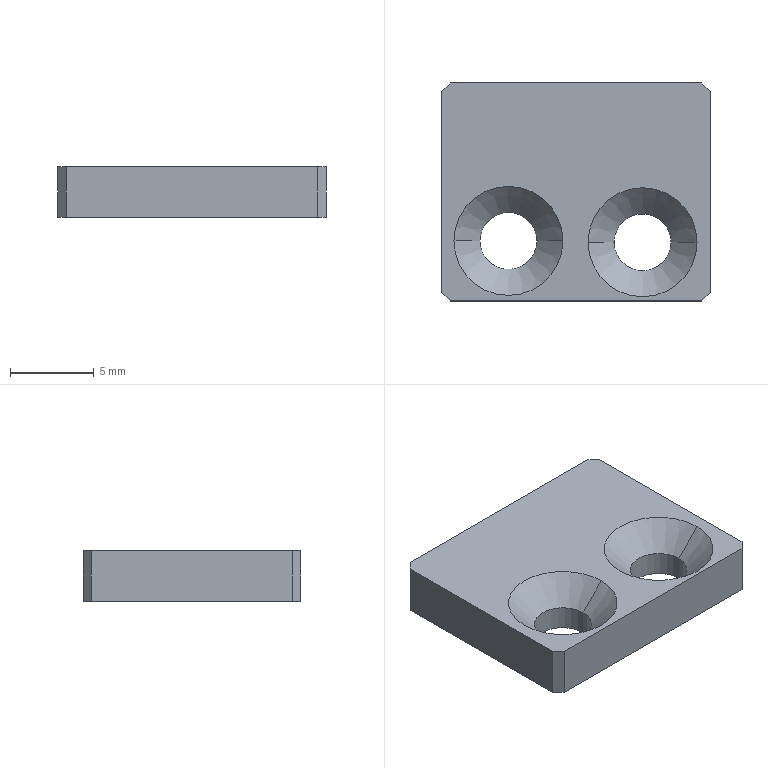Part | STEP file | 1 solid | 18 faces | box 16 x 13 x 3 mm | volume 534.563 mm3 | plane 10 | cone 4 | cylinder 4 | commonest cylinder face diameters 3.4 x4
STEP:
#1=CARTESIAN_POINT('',(0.,0.,0.));
#2=DIRECTION('',(0.,0.,1.));
#3=DIRECTION('',(1.,0.,0.));
#4=AXIS2_PLACEMENT_3D('',#1,#2,#3);
#5=CARTESIAN_POINT('',(7.5,-6.5,3.));
#6=VERTEX_POINT('',#5);
#7=CARTESIAN_POINT('',(8.,-6.,3.));
#8=VERTEX_POINT('',#7);
#9=CARTESIAN_POINT('',(8.,-6.,3.));
#10=DIRECTION('',(0.7071,0.7071,0.));
#11=VECTOR('',#10,1.);
#12=LINE('',#9,#11);
#13=CARTESIAN_POINT('',(8.,-6.,3.));
#14=DIRECTION('',(-0.7071,0.7071,0.));
#15=DIRECTION('',(0.,0.,-1.));
#16=AXIS2_PLACEMENT_3D('',#13,#14,#15);
#17=PLANE('',#16);
#18=CARTESIAN_POINT('',(0.,0.));
#19=DIRECTION('',(0.,-1.));
#20=VECTOR('',#19,1.);
#21=LINE('',#18,#20);
#22=(GEOMETRIC_REPRESENTATION_CONTEXT(2)PARAMETRIC_REPRESENTATION_CONTEXT()REPRESENTATION_CONTEXT('',''));
#23=DEFINITIONAL_REPRESENTATION('',(#21),#22);
#24=PCURVE('',#17,#23);
#25=CARTESIAN_POINT('',(0.,0.,3.));
#26=DIRECTION('',(0.,0.,-1.));
#27=DIRECTION('',(-1.,0.,0.));
#28=AXIS2_PLACEMENT_3D('',#25,#26,#27);
#29=PLANE('',#28);
#30=CARTESIAN_POINT('',(-8.,-6.));
#31=DIRECTION('',(-0.7071,0.7071));
#32=VECTOR('',#31,1.);
#33=LINE('',#30,#32);
#34=(GEOMETRIC_REPRESENTATION_CONTEXT(2)PARAMETRIC_REPRESENTATION_CONTEXT()REPRESENTATION_CONTEXT('',''));
#35=DEFINITIONAL_REPRESENTATION('',(#33),#34);
#36=PCURVE('',#29,#35);
#37=SURFACE_CURVE('',#12,(#24,#36),.PCURVE_S1.);
#38=EDGE_CURVE('',#6,#8,#37,.T.);
#39=ORIENTED_EDGE('',*,*,#38,.F.);
#40=CARTESIAN_POINT('',(7.5,-6.5,0.));
#41=VERTEX_POINT('',#40);
#42=CARTESIAN_POINT('',(7.5,-6.5,3.));
#43=DIRECTION('',(0.,0.,1.));
#44=VECTOR('',#43,1.);
#45=LINE('',#42,#44);
#46=CARTESIAN_POINT('',(0.,0.7071));
#47=DIRECTION('',(-1.,0.));
#48=VECTOR('',#47,1.);
#49=LINE('',#46,#48);
#50=(GEOMETRIC_REPRESENTATION_CONTEXT(2)PARAMETRIC_REPRESENTATION_CONTEXT()REPRESENTATION_CONTEXT('',''));
#51=DEFINITIONAL_REPRESENTATION('',(#49),#50);
#52=PCURVE('',#17,#51);
#53=CARTESIAN_POINT('',(-8.,-6.5,3.));
#54=DIRECTION('',(0.,1.,0.));
#55=DIRECTION('',(0.,0.,1.));
#56=AXIS2_PLACEMENT_3D('',#53,#54,#55);
#57=PLANE('',#56);
#58=CARTESIAN_POINT('',(0.,15.5));
#59=DIRECTION('',(1.,0.));
#60=VECTOR('',#59,1.);
#61=LINE('',#58,#60);
#62=(GEOMETRIC_REPRESENTATION_CONTEXT(2)PARAMETRIC_REPRESENTATION_CONTEXT()REPRESENTATION_CONTEXT('',''));
#63=DEFINITIONAL_REPRESENTATION('',(#61),#62);
#64=PCURVE('',#57,#63);
#65=SURFACE_CURVE('',#45,(#52,#64),.PCURVE_S1.);
#66=EDGE_CURVE('',#41,#6,#65,.T.);
#67=ORIENTED_EDGE('',*,*,#66,.F.);
#68=CARTESIAN_POINT('',(8.,-6.,0.));
#69=VERTEX_POINT('',#68);
#70=CARTESIAN_POINT('',(7.,-7.,0.));
#71=DIRECTION('',(-0.7071,-0.7071,0.));
#72=VECTOR('',#71,1.);
#73=LINE('',#70,#72);
#74=CARTESIAN_POINT('',(3.,1.414));
#75=DIRECTION('',(0.,1.));
#76=VECTOR('',#75,1.);
#77=LINE('',#74,#76);
#78=(GEOMETRIC_REPRESENTATION_CONTEXT(2)PARAMETRIC_REPRESENTATION_CONTEXT()REPRESENTATION_CONTEXT('',''));
#79=DEFINITIONAL_REPRESENTATION('',(#77),#78);
#80=PCURVE('',#17,#79);
#81=CARTESIAN_POINT('',(0.,0.,0.));
#82=DIRECTION('',(0.,0.,-1.));
#83=DIRECTION('',(-1.,0.,0.));
#84=AXIS2_PLACEMENT_3D('',#81,#82,#83);
#85=PLANE('',#84);
#86=CARTESIAN_POINT('',(-7.,-7.));
#87=DIRECTION('',(0.7071,-0.7071));
#88=VECTOR('',#87,1.);
#89=LINE('',#86,#88);
#90=(GEOMETRIC_REPRESENTATION_CONTEXT(2)PARAMETRIC_REPRESENTATION_CONTEXT()REPRESENTATION_CONTEXT('',''));
#91=DEFINITIONAL_REPRESENTATION('',(#89),#90);
#92=PCURVE('',#85,#91);
#93=SURFACE_CURVE('',#73,(#80,#92),.PCURVE_S1.);
#94=EDGE_CURVE('',#69,#41,#93,.T.);
#95=ORIENTED_EDGE('',*,*,#94,.F.);
#96=CARTESIAN_POINT('',(8.,-6.,3.));
#97=DIRECTION('',(0.,0.,-1.));
#98=VECTOR('',#97,1.);
#99=LINE('',#96,#98);
#100=CARTESIAN_POINT('',(0.,0.));
#101=DIRECTION('',(1.,0.));
#102=VECTOR('',#101,1.);
#103=LINE('',#100,#102);
#104=(GEOMETRIC_REPRESENTATION_CONTEXT(2)PARAMETRIC_REPRESENTATION_CONTEXT()REPRESENTATION_CONTEXT('',''));
#105=DEFINITIONAL_REPRESENTATION('',(#103),#104);
#106=PCURVE('',#17,#105);
#107=CARTESIAN_POINT('',(8.,-6.5,3.));
#108=DIRECTION('',(-1.,0.,0.));
#109=DIRECTION('',(0.,0.,1.));
#110=AXIS2_PLACEMENT_3D('',#107,#108,#109);
#111=PLANE('',#110);
#112=CARTESIAN_POINT('',(0.,0.5));
#113=DIRECTION('',(-1.,0.));
#114=VECTOR('',#113,1.);
#115=LINE('',#112,#114);
#116=(GEOMETRIC_REPRESENTATION_CONTEXT(2)PARAMETRIC_REPRESENTATION_CONTEXT()REPRESENTATION_CONTEXT('',''));
#117=DEFINITIONAL_REPRESENTATION('',(#115),#116);
#118=PCURVE('',#111,#117);
#119=SURFACE_CURVE('',#99,(#106,#118),.PCURVE_S1.);
#120=EDGE_CURVE('',#8,#69,#119,.T.);
#121=ORIENTED_EDGE('',*,*,#120,.F.);
#122=EDGE_LOOP('',(#39,#67,#95,#121));
#123=FACE_BOUND('',#122,.T.);
#124=ADVANCED_FACE('',(#123),#17,.F.);
#125=CARTESIAN_POINT('',(-8.,-6.,3.));
#126=VERTEX_POINT('',#125);
#127=CARTESIAN_POINT('',(-7.5,-6.5,3.));
#128=VERTEX_POINT('',#127);
#129=CARTESIAN_POINT('',(-7.5,-6.5,3.));
#130=DIRECTION('',(0.7071,-0.7071,0.));
#131=VECTOR('',#130,1.);
#132=LINE('',#129,#131);
#133=CARTESIAN_POINT('',(-7.5,-6.5,3.));
#134=DIRECTION('',(0.7071,0.7071,0.));
#135=DIRECTION('',(0.,0.,-1.));
#136=AXIS2_PLACEMENT_3D('',#133,#134,#135);
#137=PLANE('',#136);
#138=CARTESIAN_POINT('',(0.,0.));
#139=DIRECTION('',(0.,-1.));
#140=VECTOR('',#139,1.);
#141=LINE('',#138,#140);
#142=(GEOMETRIC_REPRESENTATION_CONTEXT(2)PARAMETRIC_REPRESENTATION_CONTEXT()REPRESENTATION_CONTEXT('',''));
#143=DEFINITIONAL_REPRESENTATION('',(#141),#142);
#144=PCURVE('',#137,#143);
#145=CARTESIAN_POINT('',(7.5,-6.5));
#146=DIRECTION('',(-0.7071,-0.7071));
#147=VECTOR('',#146,1.);
#148=LINE('',#145,#147);
#149=(GEOMETRIC_REPRESENTATION_CONTEXT(2)PARAMETRIC_REPRESENTATION_CONTEXT()REPRESENTATION_CONTEXT('',''));
#150=DEFINITIONAL_REPRESENTATION('',(#148),#149);
#151=PCURVE('',#29,#150);
#152=SURFACE_CURVE('',#132,(#144,#151),.PCURVE_S1.);
#153=EDGE_CURVE('',#126,#128,#152,.T.);
#154=ORIENTED_EDGE('',*,*,#153,.F.);
#155=CARTESIAN_POINT('',(-8.,-6.,0.));
#156=VERTEX_POINT('',#155);
#157=CARTESIAN_POINT('',(-8.,-6.,3.));
#158=DIRECTION('',(0.,0.,1.));
#159=VECTOR('',#158,1.);
#160=LINE('',#157,#159);
#161=CARTESIAN_POINT('',(0.,0.7071));
#162=DIRECTION('',(-1.,0.));
#163=VECTOR('',#162,1.);
#164=LINE('',#161,#163);
#165=(GEOMETRIC_REPRESENTATION_CONTEXT(2)PARAMETRIC_REPRESENTATION_CONTEXT()REPRESENTATION_CONTEXT('',''));
#166=DEFINITIONAL_REPRESENTATION('',(#164),#165);
#167=PCURVE('',#137,#166);
#168=CARTESIAN_POINT('',(-8.,-6.5,3.));
#169=DIRECTION('',(1.,0.,0.));
#170=DIRECTION('',(0.,0.,-1.));
#171=AXIS2_PLACEMENT_3D('',#168,#169,#170);
#172=PLANE('',#171);
#173=CARTESIAN_POINT('',(0.,0.5));
#174=DIRECTION('',(-1.,0.));
#175=VECTOR('',#174,1.);
#176=LINE('',#173,#175);
#177=(GEOMETRIC_REPRESENTATION_CONTEXT(2)PARAMETRIC_REPRESENTATION_CONTEXT()REPRESENTATION_CONTEXT('',''));
#178=DEFINITIONAL_REPRESENTATION('',(#176),#177);
#179=PCURVE('',#172,#178);
#180=SURFACE_CURVE('',#160,(#167,#179),.PCURVE_S1.);
#181=EDGE_CURVE('',#156,#126,#180,.T.);
#182=ORIENTED_EDGE('',*,*,#181,.F.);
#183=CARTESIAN_POINT('',(-7.5,-6.5,0.));
#184=VERTEX_POINT('',#183);
#185=CARTESIAN_POINT('',(-7.,-7.,0.));
#186=DIRECTION('',(-0.7071,0.7071,0.));
#187=VECTOR('',#186,1.);
#188=LINE('',#185,#187);
#189=CARTESIAN_POINT('',(3.,-0.7071));
#190=DIRECTION('',(0.,1.));
#191=VECTOR('',#190,1.);
#192=LINE('',#189,#191);
#193=(GEOMETRIC_REPRESENTATION_CONTEXT(2)PARAMETRIC_REPRESENTATION_CONTEXT()REPRESENTATION_CONTEXT('',''));
#194=DEFINITIONAL_REPRESENTATION('',(#192),#193);
#195=PCURVE('',#137,#194);
#196=CARTESIAN_POINT('',(7.,-7.));
#197=DIRECTION('',(0.7071,0.7071));
#198=VECTOR('',#197,1.);
#199=LINE('',#196,#198);
#200=(GEOMETRIC_REPRESENTATION_CONTEXT(2)PARAMETRIC_REPRESENTATION_CONTEXT()REPRESENTATION_CONTEXT('',''));
#201=DEFINITIONAL_REPRESENTATION('',(#199),#200);
#202=PCURVE('',#85,#201);
#203=SURFACE_CURVE('',#188,(#195,#202),.PCURVE_S1.);
#204=EDGE_CURVE('',#184,#156,#203,.T.);
#205=ORIENTED_EDGE('',*,*,#204,.F.);
#206=CARTESIAN_POINT('',(-7.5,-6.5,3.));
#207=DIRECTION('',(0.,0.,-1.));
#208=VECTOR('',#207,1.);
#209=LINE('',#206,#208);
#210=CARTESIAN_POINT('',(0.,0.));
#211=DIRECTION('',(1.,0.));
#212=VECTOR('',#211,1.);
#213=LINE('',#210,#212);
#214=(GEOMETRIC_REPRESENTATION_CONTEXT(2)PARAMETRIC_REPRESENTATION_CONTEXT()REPRESENTATION_CONTEXT('',''));
#215=DEFINITIONAL_REPRESENTATION('',(#213),#214);
#216=PCURVE('',#137,#215);
#217=CARTESIAN_POINT('',(0.,0.5));
#218=DIRECTION('',(-1.,0.));
#219=VECTOR('',#218,1.);
#220=LINE('',#217,#219);
#221=(GEOMETRIC_REPRESENTATION_CONTEXT(2)PARAMETRIC_REPRESENTATION_CONTEXT()REPRESENTATION_CONTEXT('',''));
#222=DEFINITIONAL_REPRESENTATION('',(#220),#221);
#223=PCURVE('',#57,#222);
#224=SURFACE_CURVE('',#209,(#216,#223),.PCURVE_S1.);
#225=EDGE_CURVE('',#128,#184,#224,.T.);
#226=ORIENTED_EDGE('',*,*,#225,.F.);
#227=EDGE_LOOP('',(#154,#182,#205,#226));
#228=FACE_BOUND('',#227,.T.);
#229=ADVANCED_FACE('',(#228),#137,.F.);
#230=CARTESIAN_POINT('',(-7.5,6.5,3.));
#231=VERTEX_POINT('',#230);
#232=CARTESIAN_POINT('',(-8.,6.,3.));
#233=VERTEX_POINT('',#232);
#234=CARTESIAN_POINT('',(-8.,6.,3.));
#235=DIRECTION('',(-0.7071,-0.7071,0.));
#236=VECTOR('',#235,1.);
#237=LINE('',#234,#236);
#238=CARTESIAN_POINT('',(-8.,6.,3.));
#239=DIRECTION('',(0.7071,-0.7071,0.));
#240=DIRECTION('',(0.,0.,-1.));
#241=AXIS2_PLACEMENT_3D('',#238,#239,#240);
#242=PLANE('',#241);
#243=CARTESIAN_POINT('',(0.,0.));
#244=DIRECTION('',(0.,-1.));
#245=VECTOR('',#244,1.);
#246=LINE('',#243,#245);
#247=(GEOMETRIC_REPRESENTATION_CONTEXT(2)PARAMETRIC_REPRESENTATION_CONTEXT()REPRESENTATION_CONTEXT('',''));
#248=DEFINITIONAL_REPRESENTATION('',(#246),#247);
#249=PCURVE('',#242,#248);
#250=CARTESIAN_POINT('',(8.,6.));
#251=DIRECTION('',(0.7071,-0.7071));
#252=VECTOR('',#251,1.);
#253=LINE('',#250,#252);
#254=(GEOMETRIC_REPRESENTATION_CONTEXT(2)PARAMETRIC_REPRESENTATION_CONTEXT()REPRESENTATION_CONTEXT('',''));
#255=DEFINITIONAL_REPRESENTATION('',(#253),#254);
#256=PCURVE('',#29,#255);
#257=SURFACE_CURVE('',#237,(#249,#256),.PCURVE_S1.);
#258=EDGE_CURVE('',#231,#233,#257,.T.);
#259=ORIENTED_EDGE('',*,*,#258,.F.);
#260=CARTESIAN_POINT('',(-7.5,6.5,0.));
#261=VERTEX_POINT('',#260);
#262=CARTESIAN_POINT('',(-7.5,6.5,3.));
#263=DIRECTION('',(0.,0.,1.));
#264=VECTOR('',#263,1.);
#265=LINE('',#262,#264);
#266=CARTESIAN_POINT('',(0.,0.7071));
#267=DIRECTION('',(-1.,0.));
#268=VECTOR('',#267,1.);
#269=LINE('',#266,#268);
#270=(GEOMETRIC_REPRESENTATION_CONTEXT(2)PARAMETRIC_REPRESENTATION_CONTEXT()REPRESENTATION_CONTEXT('',''));
#271=DEFINITIONAL_REPRESENTATION('',(#269),#270);
#272=PCURVE('',#242,#271);
#273=CARTESIAN_POINT('',(-8.,6.5,3.));
#274=DIRECTION('',(0.,-1.,0.));
#275=DIRECTION('',(0.,0.,-1.));
#276=AXIS2_PLACEMENT_3D('',#273,#274,#275);
#277=PLANE('',#276);
#278=CARTESIAN_POINT('',(0.,0.5));
#279=DIRECTION('',(-1.,0.));
#280=VECTOR('',#279,1.);
#281=LINE('',#278,#280);
#282=(GEOMETRIC_REPRESENTATION_CONTEXT(2)PARAMETRIC_REPRESENTATION_CONTEXT()REPRESENTATION_CONTEXT('',''));
#283=DEFINITIONAL_REPRESENTATION('',(#281),#282);
#284=PCURVE('',#277,#283);
#285=SURFACE_CURVE('',#265,(#272,#284),.PCURVE_S1.);
#286=EDGE_CURVE('',#261,#231,#285,.T.);
#287=ORIENTED_EDGE('',*,*,#286,.F.);
#288=CARTESIAN_POINT('',(-8.,6.,0.));
#289=VERTEX_POINT('',#288);
#290=CARTESIAN_POINT('',(-7.,7.,0.));
#291=DIRECTION('',(0.7071,0.7071,0.));
#292=VECTOR('',#291,1.);
#293=LINE('',#290,#292);
#294=CARTESIAN_POINT('',(3.,1.414));
#295=DIRECTION('',(0.,1.));
#296=VECTOR('',#295,1.);
#297=LINE('',#294,#296);
#298=(GEOMETRIC_REPRESENTATION_CONTEXT(2)PARAMETRIC_REPRESENTATION_CONTEXT()REPRESENTATION_CONTEXT('',''));
#299=DEFINITIONAL_REPRESENTATION('',(#297),#298);
#300=PCURVE('',#242,#299);
#301=CARTESIAN_POINT('',(7.,7.));
#302=DIRECTION('',(-0.7071,0.7071));
#303=VECTOR('',#302,1.);
#304=LINE('',#301,#303);
#305=(GEOMETRIC_REPRESENTATION_CONTEXT(2)PARAMETRIC_REPRESENTATION_CONTEXT()REPRESENTATION_CONTEXT('',''));
#306=DEFINITIONAL_REPRESENTATION('',(#304),#305);
#307=PCURVE('',#85,#306);
#308=SURFACE_CURVE('',#293,(#300,#307),.PCURVE_S1.);
#309=EDGE_CURVE('',#289,#261,#308,.T.);
#310=ORIENTED_EDGE('',*,*,#309,.F.);
#311=CARTESIAN_POINT('',(-8.,6.,3.));
#312=DIRECTION('',(0.,0.,-1.));
#313=VECTOR('',#312,1.);
#314=LINE('',#311,#313);
#315=CARTESIAN_POINT('',(0.,0.));
#316=DIRECTION('',(1.,0.));
#317=VECTOR('',#316,1.);
#318=LINE('',#315,#317);
#319=(GEOMETRIC_REPRESENTATION_CONTEXT(2)PARAMETRIC_REPRESENTATION_CONTEXT()REPRESENTATION_CONTEXT('',''));
#320=DEFINITIONAL_REPRESENTATION('',(#318),#319);
#321=PCURVE('',#242,#320);
#322=CARTESIAN_POINT('',(0.,12.5));
#323=DIRECTION('',(1.,0.));
#324=VECTOR('',#323,1.);
#325=LINE('',#322,#324);
#326=(GEOMETRIC_REPRESENTATION_CONTEXT(2)PARAMETRIC_REPRESENTATION_CONTEXT()REPRESENTATION_CONTEXT('',''));
#327=DEFINITIONAL_REPRESENTATION('',(#325),#326);
#328=PCURVE('',#172,#327);
#329=SURFACE_CURVE('',#314,(#321,#328),.PCURVE_S1.);
#330=EDGE_CURVE('',#233,#289,#329,.T.);
#331=ORIENTED_EDGE('',*,*,#330,.F.);
#332=EDGE_LOOP('',(#259,#287,#310,#331));
#333=FACE_BOUND('',#332,.T.);
#334=ADVANCED_FACE('',(#333),#242,.F.);
#335=CARTESIAN_POINT('',(8.,6.,3.));
#336=VERTEX_POINT('',#335);
#337=CARTESIAN_POINT('',(7.5,6.5,3.));
#338=VERTEX_POINT('',#337);
#339=CARTESIAN_POINT('',(7.5,6.5,3.));
#340=DIRECTION('',(-0.7071,0.7071,0.));
#341=VECTOR('',#340,1.);
#342=LINE('',#339,#341);
#343=CARTESIAN_POINT('',(7.5,6.5,3.));
#344=DIRECTION('',(-0.7071,-0.7071,0.));
#345=DIRECTION('',(0.,0.,-1.));
#346=AXIS2_PLACEMENT_3D('',#343,#344,#345);
#347=PLANE('',#346);
#348=CARTESIAN_POINT('',(0.,0.));
#349=DIRECTION('',(0.,-1.));
#350=VECTOR('',#349,1.);
#351=LINE('',#348,#350);
#352=(GEOMETRIC_REPRESENTATION_CONTEXT(2)PARAMETRIC_REPRESENTATION_CONTEXT()REPRESENTATION_CONTEXT('',''));
#353=DEFINITIONAL_REPRESENTATION('',(#351),#352);
#354=PCURVE('',#347,#353);
#355=CARTESIAN_POINT('',(-7.5,6.5));
#356=DIRECTION('',(0.7071,0.7071));
#357=VECTOR('',#356,1.);
#358=LINE('',#355,#357);
#359=(GEOMETRIC_REPRESENTATION_CONTEXT(2)PARAMETRIC_REPRESENTATION_CONTEXT()REPRESENTATION_CONTEXT('',''));
#360=DEFINITIONAL_REPRESENTATION('',(#358),#359);
#361=PCURVE('',#29,#360);
#362=SURFACE_CURVE('',#342,(#354,#361),.PCURVE_S1.);
#363=EDGE_CURVE('',#336,#338,#362,.T.);
#364=ORIENTED_EDGE('',*,*,#363,.F.);
#365=CARTESIAN_POINT('',(8.,6.,0.));
#366=VERTEX_POINT('',#365);
#367=CARTESIAN_POINT('',(8.,6.,3.));
#368=DIRECTION('',(0.,0.,1.));
#369=VECTOR('',#368,1.);
#370=LINE('',#367,#369);
#371=CARTESIAN_POINT('',(0.,0.7071));
#372=DIRECTION('',(-1.,0.));
#373=VECTOR('',#372,1.);
#374=LINE('',#371,#373);
#375=(GEOMETRIC_REPRESENTATION_CONTEXT(2)PARAMETRIC_REPRESENTATION_CONTEXT()REPRESENTATION_CONTEXT('',''));
#376=DEFINITIONAL_REPRESENTATION('',(#374),#375);
#377=PCURVE('',#347,#376);
#378=CARTESIAN_POINT('',(0.,12.5));
#379=DIRECTION('',(1.,0.));
#380=VECTOR('',#379,1.);
#381=LINE('',#378,#380);
#382=(GEOMETRIC_REPRESENTATION_CONTEXT(2)PARAMETRIC_REPRESENTATION_CONTEXT()REPRESENTATION_CONTEXT('',''));
#383=DEFINITIONAL_REPRESENTATION('',(#381),#382);
#384=PCURVE('',#111,#383);
#385=SURFACE_CURVE('',#370,(#377,#384),.PCURVE_S1.);
#386=EDGE_CURVE('',#366,#336,#385,.T.);
#387=ORIENTED_EDGE('',*,*,#386,.F.);
#388=CARTESIAN_POINT('',(7.5,6.5,0.));
#389=VERTEX_POINT('',#388);
#390=CARTESIAN_POINT('',(7.,7.,0.));
#391=DIRECTION('',(0.7071,-0.7071,0.));
#392=VECTOR('',#391,1.);
#393=LINE('',#390,#392);
#394=CARTESIAN_POINT('',(3.,-0.7071));
#395=DIRECTION('',(0.,1.));
#396=VECTOR('',#395,1.);
#397=LINE('',#394,#396);
#398=(GEOMETRIC_REPRESENTATION_CONTEXT(2)PARAMETRIC_REPRESENTATION_CONTEXT()REPRESENTATION_CONTEXT('',''));
#399=DEFINITIONAL_REPRESENTATION('',(#397),#398);
#400=PCURVE('',#347,#399);
#401=CARTESIAN_POINT('',(-7.,7.));
#402=DIRECTION('',(-0.7071,-0.7071));
#403=VECTOR('',#402,1.);
#404=LINE('',#401,#403);
#405=(GEOMETRIC_REPRESENTATION_CONTEXT(2)PARAMETRIC_REPRESENTATION_CONTEXT()REPRESENTATION_CONTEXT('',''));
#406=DEFINITIONAL_REPRESENTATION('',(#404),#405);
#407=PCURVE('',#85,#406);
#408=SURFACE_CURVE('',#393,(#400,#407),.PCURVE_S1.);
#409=EDGE_CURVE('',#389,#366,#408,.T.);
#410=ORIENTED_EDGE('',*,*,#409,.F.);
#411=CARTESIAN_POINT('',(7.5,6.5,3.));
#412=DIRECTION('',(0.,0.,-1.));
#413=VECTOR('',#412,1.);
#414=LINE('',#411,#413);
#415=CARTESIAN_POINT('',(0.,0.));
#416=DIRECTION('',(1.,0.));
#417=VECTOR('',#416,1.);
#418=LINE('',#415,#417);
#419=(GEOMETRIC_REPRESENTATION_CONTEXT(2)PARAMETRIC_REPRESENTATION_CONTEXT()REPRESENTATION_CONTEXT('',''));
#420=DEFINITIONAL_REPRESENTATION('',(#418),#419);
#421=PCURVE('',#347,#420);
#422=CARTESIAN_POINT('',(0.,15.5));
#423=DIRECTION('',(1.,0.));
#424=VECTOR('',#423,1.);
#425=LINE('',#422,#424);
#426=(GEOMETRIC_REPRESENTATION_CONTEXT(2)PARAMETRIC_REPRESENTATION_CONTEXT()REPRESENTATION_CONTEXT('',''));
#427=DEFINITIONAL_REPRESENTATION('',(#425),#426);
#428=PCURVE('',#277,#427);
#429=SURFACE_CURVE('',#414,(#421,#428),.PCURVE_S1.);
#430=EDGE_CURVE('',#338,#389,#429,.T.);
#431=ORIENTED_EDGE('',*,*,#430,.F.);
#432=EDGE_LOOP('',(#364,#387,#410,#431));
#433=FACE_BOUND('',#432,.T.);
#434=ADVANCED_FACE('',(#433),#347,.F.);
#435=CARTESIAN_POINT('',(-0.7797,-2.919,3.));
#436=VERTEX_POINT('',#435);
#437=CARTESIAN_POINT('',(-7.28,-2.919,3.));
#438=VERTEX_POINT('',#437);
#439=CARTESIAN_POINT('',(-4.03,-2.919,3.));
#440=DIRECTION('',(0.,0.,1.));
#441=DIRECTION('',(1.,0.,0.));
#442=AXIS2_PLACEMENT_3D('',#439,#440,#441);
#443=CIRCLE('',#442,3.25);
#444=CARTESIAN_POINT('',(-4.03,-2.919,3.));
#445=DIRECTION('',(0.,0.,1.));
#446=DIRECTION('',(1.,0.,0.));
#447=AXIS2_PLACEMENT_3D('',#444,#445,#446);
#448=CONICAL_SURFACE('',#447,3.25,0.7854);
#449=CARTESIAN_POINT('',(0.,0.));
#450=DIRECTION('',(1.,0.));
#451=VECTOR('',#450,1.);
#452=LINE('',#449,#451);
#453=(GEOMETRIC_REPRESENTATION_CONTEXT(2)PARAMETRIC_REPRESENTATION_CONTEXT()REPRESENTATION_CONTEXT('',''));
#454=DEFINITIONAL_REPRESENTATION('',(#452),#453);
#455=PCURVE('',#448,#454);
#456=CARTESIAN_POINT('',(0.7797,-2.919));
#457=CARTESIAN_POINT('',(0.7797,2.71));
#458=CARTESIAN_POINT('',(5.655,-0.1046));
#459=CARTESIAN_POINT('',(10.53,-2.919));
#460=CARTESIAN_POINT('',(5.655,-5.734));
#461=CARTESIAN_POINT('',(0.7797,-8.548));
#462=CARTESIAN_POINT('',(0.7797,-2.919));
#463=(BOUNDED_CURVE()B_SPLINE_CURVE(2,(#456,#457,#458,#459,#460,#461,#462),.UNSPECIFIED.,.T.,.F.)B_SPLINE_CURVE_WITH_KNOTS((1,2,2,2,2,1),(-2.094,0.,2.094,4.189,6.283,8.378),.UNSPECIFIED.)CURVE()GEOMETRIC_REPRESENTATION_ITEM()RATIONAL_B_SPLINE_CURVE((1.,0.5,1.,0.5,1.,0.5,1.))REPRESENTATION_ITEM(''));
#464=(GEOMETRIC_REPRESENTATION_CONTEXT(2)PARAMETRIC_REPRESENTATION_CONTEXT()REPRESENTATION_CONTEXT('',''));
#465=DEFINITIONAL_REPRESENTATION('',(#463),#464);
#466=PCURVE('',#29,#465);
#467=SURFACE_CURVE('',#443,(#455,#466),.PCURVE_S1.);
#468=EDGE_CURVE('',#436,#438,#467,.T.);
#469=ORIENTED_EDGE('',*,*,#468,.F.);
#470=CARTESIAN_POINT('',(-2.33,-2.919,1.45));
#471=VERTEX_POINT('',#470);
#472=CARTESIAN_POINT('',(-0.7797,-2.919,3.));
#473=DIRECTION('',(0.7071,0.,0.7071));
#474=VECTOR('',#473,1.);
#475=LINE('',#472,#474);
#476=CARTESIAN_POINT('',(0.,0.));
#477=DIRECTION('',(0.,1.));
#478=VECTOR('',#477,1.);
#479=LINE('',#476,#478);
#480=(GEOMETRIC_REPRESENTATION_CONTEXT(2)PARAMETRIC_REPRESENTATION_CONTEXT()REPRESENTATION_CONTEXT('',''));
#481=DEFINITIONAL_REPRESENTATION('',(#479),#480);
#482=PCURVE('',#448,#481);
#483=CARTESIAN_POINT('',(-4.03,-2.919,3.));
#484=DIRECTION('',(0.,0.,1.));
#485=DIRECTION('',(1.,0.,0.));
#486=AXIS2_PLACEMENT_3D('',#483,#484,#485);
#487=CONICAL_SURFACE('',#486,3.25,0.7854);
#488=CARTESIAN_POINT('',(6.283,0.));
#489=DIRECTION('',(0.,1.));
#490=VECTOR('',#489,1.);
#491=LINE('',#488,#490);
#492=(GEOMETRIC_REPRESENTATION_CONTEXT(2)PARAMETRIC_REPRESENTATION_CONTEXT()REPRESENTATION_CONTEXT('',''));
#493=DEFINITIONAL_REPRESENTATION('',(#491),#492);
#494=PCURVE('',#487,#493);
#495=SURFACE_CURVE('',#475,(#482,#494),.PCURVE_S1.);
#496=EDGE_CURVE('',#471,#436,#495,.T.);
#497=ORIENTED_EDGE('',*,*,#496,.F.);
#498=CARTESIAN_POINT('',(-5.73,-2.919,1.45));
#499=VERTEX_POINT('',#498);
#500=CARTESIAN_POINT('',(-4.03,-2.919,1.45));
#501=DIRECTION('',(0.,0.,1.));
#502=DIRECTION('',(1.,0.,0.));
#503=AXIS2_PLACEMENT_3D('',#500,#501,#502);
#504=CIRCLE('',#503,1.7);
#505=CARTESIAN_POINT('',(0.,-1.55));
#506=DIRECTION('',(1.,0.));
#507=VECTOR('',#506,1.);
#508=LINE('',#505,#507);
#509=(GEOMETRIC_REPRESENTATION_CONTEXT(2)PARAMETRIC_REPRESENTATION_CONTEXT()REPRESENTATION_CONTEXT('',''));
#510=DEFINITIONAL_REPRESENTATION('',(#508),#509);
#511=PCURVE('',#448,#510);
#512=CARTESIAN_POINT('',(-4.03,-2.919,3.));
#513=DIRECTION('',(0.,0.,1.));
#514=DIRECTION('',(1.,0.,0.));
#515=AXIS2_PLACEMENT_3D('',#512,#513,#514);
#516=CYLINDRICAL_SURFACE('',#515,1.7);
#517=CARTESIAN_POINT('',(0.,-1.55));
#518=DIRECTION('',(1.,0.));
#519=VECTOR('',#518,1.);
#520=LINE('',#517,#519);
#521=(GEOMETRIC_REPRESENTATION_CONTEXT(2)PARAMETRIC_REPRESENTATION_CONTEXT()REPRESENTATION_CONTEXT('',''));
#522=DEFINITIONAL_REPRESENTATION('',(#520),#521);
#523=PCURVE('',#516,#522);
#524=SURFACE_CURVE('',#504,(#511,#523),.PCURVE_S1.);
#525=EDGE_CURVE('',#471,#499,#524,.T.);
#526=ORIENTED_EDGE('',*,*,#525,.T.);
#527=CARTESIAN_POINT('',(-7.28,-2.919,3.));
#528=DIRECTION('',(-0.7071,0.,0.7071));
#529=VECTOR('',#528,1.);
#530=LINE('',#527,#529);
#531=CARTESIAN_POINT('',(3.142,0.));
#532=DIRECTION('',(0.,1.));
#533=VECTOR('',#532,1.);
#534=LINE('',#531,#533);
#535=(GEOMETRIC_REPRESENTATION_CONTEXT(2)PARAMETRIC_REPRESENTATION_CONTEXT()REPRESENTATION_CONTEXT('',''));
#536=DEFINITIONAL_REPRESENTATION('',(#534),#535);
#537=PCURVE('',#448,#536);
#538=CARTESIAN_POINT('',(3.142,0.));
#539=DIRECTION('',(0.,1.));
#540=VECTOR('',#539,1.);
#541=LINE('',#538,#540);
#542=(GEOMETRIC_REPRESENTATION_CONTEXT(2)PARAMETRIC_REPRESENTATION_CONTEXT()REPRESENTATION_CONTEXT('',''));
#543=DEFINITIONAL_REPRESENTATION('',(#541),#542);
#544=PCURVE('',#487,#543);
#545=SURFACE_CURVE('',#530,(#537,#544),.PCURVE_S1.);
#546=EDGE_CURVE('',#499,#438,#545,.T.);
#547=ORIENTED_EDGE('',*,*,#546,.T.);
#548=EDGE_LOOP('',(#469,#497,#526,#547));
#549=FACE_BOUND('',#548,.F.);
#550=ADVANCED_FACE('',(#549),#448,.F.);
#551=ORIENTED_EDGE('',*,*,#525,.F.);
#552=CARTESIAN_POINT('',(-2.33,-2.919,0.));
#553=VERTEX_POINT('',#552);
#554=CARTESIAN_POINT('',(-2.33,-2.919,3.));
#555=DIRECTION('',(0.,0.,1.));
#556=VECTOR('',#555,1.);
#557=LINE('',#554,#556);
#558=CARTESIAN_POINT('',(0.,0.));
#559=DIRECTION('',(0.,1.));
#560=VECTOR('',#559,1.);
#561=LINE('',#558,#560);
#562=(GEOMETRIC_REPRESENTATION_CONTEXT(2)PARAMETRIC_REPRESENTATION_CONTEXT()REPRESENTATION_CONTEXT('',''));
#563=DEFINITIONAL_REPRESENTATION('',(#561),#562);
#564=PCURVE('',#516,#563);
#565=CARTESIAN_POINT('',(-4.03,-2.919,3.));
#566=DIRECTION('',(0.,0.,1.));
#567=DIRECTION('',(1.,0.,0.));
#568=AXIS2_PLACEMENT_3D('',#565,#566,#567);
#569=CYLINDRICAL_SURFACE('',#568,1.7);
#570=CARTESIAN_POINT('',(6.283,0.));
#571=DIRECTION('',(0.,1.));
#572=VECTOR('',#571,1.);
#573=LINE('',#570,#572);
#574=(GEOMETRIC_REPRESENTATION_CONTEXT(2)PARAMETRIC_REPRESENTATION_CONTEXT()REPRESENTATION_CONTEXT('',''));
#575=DEFINITIONAL_REPRESENTATION('',(#573),#574);
#576=PCURVE('',#569,#575);
#577=SURFACE_CURVE('',#557,(#564,#576),.PCURVE_S1.);
#578=EDGE_CURVE('',#553,#471,#577,.T.);
#579=ORIENTED_EDGE('',*,*,#578,.F.);
#580=CARTESIAN_POINT('',(-5.73,-2.919,0.));
#581=VERTEX_POINT('',#580);
#582=CARTESIAN_POINT('',(-4.03,-2.919,0.));
#583=DIRECTION('',(0.,0.,1.));
#584=DIRECTION('',(1.,0.,0.));
#585=AXIS2_PLACEMENT_3D('',#582,#583,#584);
#586=CIRCLE('',#585,1.7);
#587=CARTESIAN_POINT('',(0.,-3.));
#588=DIRECTION('',(1.,0.));
#589=VECTOR('',#588,1.);
#590=LINE('',#587,#589);
#591=(GEOMETRIC_REPRESENTATION_CONTEXT(2)PARAMETRIC_REPRESENTATION_CONTEXT()REPRESENTATION_CONTEXT('',''));
#592=DEFINITIONAL_REPRESENTATION('',(#590),#591);
#593=PCURVE('',#516,#592);
#594=CARTESIAN_POINT('',(2.33,-2.919));
#595=CARTESIAN_POINT('',(2.33,0.02529));
#596=CARTESIAN_POINT('',(4.88,-1.447));
#597=CARTESIAN_POINT('',(7.43,-2.919));
#598=CARTESIAN_POINT('',(4.88,-4.391));
#599=CARTESIAN_POINT('',(2.33,-5.864));
#600=CARTESIAN_POINT('',(2.33,-2.919));
#601=(BOUNDED_CURVE()B_SPLINE_CURVE(2,(#594,#595,#596,#597,#598,#599,#600),.UNSPECIFIED.,.T.,.F.)B_SPLINE_CURVE_WITH_KNOTS((1,2,2,2,2,1),(-2.094,0.,2.094,4.189,6.283,8.378),.UNSPECIFIED.)CURVE()GEOMETRIC_REPRESENTATION_ITEM()RATIONAL_B_SPLINE_CURVE((1.,0.5,1.,0.5,1.,0.5,1.))REPRESENTATION_ITEM(''));
#602=(GEOMETRIC_REPRESENTATION_CONTEXT(2)PARAMETRIC_REPRESENTATION_CONTEXT()REPRESENTATION_CONTEXT('',''));
#603=DEFINITIONAL_REPRESENTATION('',(#601),#602);
#604=PCURVE('',#85,#603);
#605=SURFACE_CURVE('',#586,(#593,#604),.PCURVE_S1.);
#606=EDGE_CURVE('',#553,#581,#605,.T.);
#607=ORIENTED_EDGE('',*,*,#606,.T.);
#608=CARTESIAN_POINT('',(-5.73,-2.919,3.));
#609=DIRECTION('',(0.,0.,1.));
#610=VECTOR('',#609,1.);
#611=LINE('',#608,#610);
#612=CARTESIAN_POINT('',(3.142,0.));
#613=DIRECTION('',(0.,1.));
#614=VECTOR('',#613,1.);
#615=LINE('',#612,#614);
#616=(GEOMETRIC_REPRESENTATION_CONTEXT(2)PARAMETRIC_REPRESENTATION_CONTEXT()REPRESENTATION_CONTEXT('',''));
#617=DEFINITIONAL_REPRESENTATION('',(#615),#616);
#618=PCURVE('',#516,#617);
#619=CARTESIAN_POINT('',(3.142,0.));
#620=DIRECTION('',(0.,1.));
#621=VECTOR('',#620,1.);
#622=LINE('',#619,#621);
#623=(GEOMETRIC_REPRESENTATION_CONTEXT(2)PARAMETRIC_REPRESENTATION_CONTEXT()REPRESENTATION_CONTEXT('',''));
#624=DEFINITIONAL_REPRESENTATION('',(#622),#623);
#625=PCURVE('',#569,#624);
#626=SURFACE_CURVE('',#611,(#618,#625),.PCURVE_S1.);
#627=EDGE_CURVE('',#581,#499,#626,.T.);
#628=ORIENTED_EDGE('',*,*,#627,.T.);
#629=EDGE_LOOP('',(#551,#579,#607,#628));
#630=FACE_BOUND('',#629,.F.);
#631=ADVANCED_FACE('',(#630),#516,.F.);
#632=CARTESIAN_POINT('',(7.22,-3.,3.));
#633=VERTEX_POINT('',#632);
#634=CARTESIAN_POINT('',(0.7199,-3.,3.));
#635=VERTEX_POINT('',#634);
#636=CARTESIAN_POINT('',(3.97,-3.,3.));
#637=DIRECTION('',(0.,0.,1.));
#638=DIRECTION('',(1.,0.,0.));
#639=AXIS2_PLACEMENT_3D('',#636,#637,#638);
#640=CIRCLE('',#639,3.25);
#641=CARTESIAN_POINT('',(3.97,-3.,3.));
#642=DIRECTION('',(0.,0.,1.));
#643=DIRECTION('',(1.,0.,0.));
#644=AXIS2_PLACEMENT_3D('',#641,#642,#643);
#645=CONICAL_SURFACE('',#644,3.25,0.7854);
#646=CARTESIAN_POINT('',(0.,0.));
#647=DIRECTION('',(1.,0.));
#648=VECTOR('',#647,1.);
#649=LINE('',#646,#648);
#650=(GEOMETRIC_REPRESENTATION_CONTEXT(2)PARAMETRIC_REPRESENTATION_CONTEXT()REPRESENTATION_CONTEXT('',''));
#651=DEFINITIONAL_REPRESENTATION('',(#649),#650);
#652=PCURVE('',#645,#651);
#653=CARTESIAN_POINT('',(-7.22,-3.));
#654=CARTESIAN_POINT('',(-7.22,2.629));
#655=CARTESIAN_POINT('',(-2.345,-0.1854));
#656=CARTESIAN_POINT('',(2.53,-3.));
#657=CARTESIAN_POINT('',(-2.345,-5.815));
#658=CARTESIAN_POINT('',(-7.22,-8.629));
#659=CARTESIAN_POINT('',(-7.22,-3.));
#660=(BOUNDED_CURVE()B_SPLINE_CURVE(2,(#653,#654,#655,#656,#657,#658,#659),.UNSPECIFIED.,.T.,.F.)B_SPLINE_CURVE_WITH_KNOTS((1,2,2,2,2,1),(-2.094,0.,2.094,4.189,6.283,8.378),.UNSPECIFIED.)CURVE()GEOMETRIC_REPRESENTATION_ITEM()RATIONAL_B_SPLINE_CURVE((1.,0.5,1.,0.5,1.,0.5,1.))REPRESENTATION_ITEM(''));
#661=(GEOMETRIC_REPRESENTATION_CONTEXT(2)PARAMETRIC_REPRESENTATION_CONTEXT()REPRESENTATION_CONTEXT('',''));
#662=DEFINITIONAL_REPRESENTATION('',(#660),#661);
#663=PCURVE('',#29,#662);
#664=SURFACE_CURVE('',#640,(#652,#663),.PCURVE_S1.);
#665=EDGE_CURVE('',#633,#635,#664,.T.);
#666=ORIENTED_EDGE('',*,*,#665,.F.);
#667=CARTESIAN_POINT('',(5.67,-3.,1.45));
#668=VERTEX_POINT('',#667);
#669=CARTESIAN_POINT('',(7.22,-3.,3.));
#670=DIRECTION('',(0.7071,0.,0.7071));
#671=VECTOR('',#670,1.);
#672=LINE('',#669,#671);
#673=CARTESIAN_POINT('',(0.,0.));
#674=DIRECTION('',(0.,1.));
#675=VECTOR('',#674,1.);
#676=LINE('',#673,#675);
#677=(GEOMETRIC_REPRESENTATION_CONTEXT(2)PARAMETRIC_REPRESENTATION_CONTEXT()REPRESENTATION_CONTEXT('',''));
#678=DEFINITIONAL_REPRESENTATION('',(#676),#677);
#679=PCURVE('',#645,#678);
#680=CARTESIAN_POINT('',(3.97,-3.,3.));
#681=DIRECTION('',(0.,0.,1.));
#682=DIRECTION('',(1.,0.,0.));
#683=AXIS2_PLACEMENT_3D('',#680,#681,#682);
#684=CONICAL_SURFACE('',#683,3.25,0.7854);
#685=CARTESIAN_POINT('',(6.283,0.));
#686=DIRECTION('',(0.,1.));
#687=VECTOR('',#686,1.);
#688=LINE('',#685,#687);
#689=(GEOMETRIC_REPRESENTATION_CONTEXT(2)PARAMETRIC_REPRESENTATION_CONTEXT()REPRESENTATION_CONTEXT('',''));
#690=DEFINITIONAL_REPRESENTATION('',(#688),#689);
#691=PCURVE('',#684,#690);
#692=SURFACE_CURVE('',#672,(#679,#691),.PCURVE_S1.);
#693=EDGE_CURVE('',#668,#633,#692,.T.);
#694=ORIENTED_EDGE('',*,*,#693,.F.);
#695=CARTESIAN_POINT('',(2.27,-3.,1.45));
#696=VERTEX_POINT('',#695);
#697=CARTESIAN_POINT('',(3.97,-3.,1.45));
#698=DIRECTION('',(0.,0.,1.));
#699=DIRECTION('',(1.,0.,0.));
#700=AXIS2_PLACEMENT_3D('',#697,#698,#699);
#701=CIRCLE('',#700,1.7);
#702=CARTESIAN_POINT('',(0.,-1.55));
#703=DIRECTION('',(1.,0.));
#704=VECTOR('',#703,1.);
#705=LINE('',#702,#704);
#706=(GEOMETRIC_REPRESENTATION_CONTEXT(2)PARAMETRIC_REPRESENTATION_CONTEXT()REPRESENTATION_CONTEXT('',''));
#707=DEFINITIONAL_REPRESENTATION('',(#705),#706);
#708=PCURVE('',#645,#707);
#709=CARTESIAN_POINT('',(3.97,-3.,3.));
#710=DIRECTION('',(0.,0.,1.));
#711=DIRECTION('',(1.,0.,0.));
#712=AXIS2_PLACEMENT_3D('',#709,#710,#711);
#713=CYLINDRICAL_SURFACE('',#712,1.7);
#714=CARTESIAN_POINT('',(0.,-1.55));
#715=DIRECTION('',(1.,0.));
#716=VECTOR('',#715,1.);
#717=LINE('',#714,#716);
#718=(GEOMETRIC_REPRESENTATION_CONTEXT(2)PARAMETRIC_REPRESENTATION_CONTEXT()REPRESENTATION_CONTEXT('',''));
#719=DEFINITIONAL_REPRESENTATION('',(#717),#718);
#720=PCURVE('',#713,#719);
#721=SURFACE_CURVE('',#701,(#708,#720),.PCURVE_S1.);
#722=EDGE_CURVE('',#668,#696,#721,.T.);
#723=ORIENTED_EDGE('',*,*,#722,.T.);
#724=CARTESIAN_POINT('',(0.7199,-3.,3.));
#725=DIRECTION('',(-0.7071,0.,0.7071));
#726=VECTOR('',#725,1.);
#727=LINE('',#724,#726);
#728=CARTESIAN_POINT('',(3.142,0.));
#729=DIRECTION('',(0.,1.));
#730=VECTOR('',#729,1.);
#731=LINE('',#728,#730);
#732=(GEOMETRIC_REPRESENTATION_CONTEXT(2)PARAMETRIC_REPRESENTATION_CONTEXT()REPRESENTATION_CONTEXT('',''));
#733=DEFINITIONAL_REPRESENTATION('',(#731),#732);
#734=PCURVE('',#645,#733);
#735=CARTESIAN_POINT('',(3.142,0.));
#736=DIRECTION('',(0.,1.));
#737=VECTOR('',#736,1.);
#738=LINE('',#735,#737);
#739=(GEOMETRIC_REPRESENTATION_CONTEXT(2)PARAMETRIC_REPRESENTATION_CONTEXT()REPRESENTATION_CONTEXT('',''));
#740=DEFINITIONAL_REPRESENTATION('',(#738),#739);
#741=PCURVE('',#684,#740);
#742=SURFACE_CURVE('',#727,(#734,#741),.PCURVE_S1.);
#743=EDGE_CURVE('',#696,#635,#742,.T.);
#744=ORIENTED_EDGE('',*,*,#743,.T.);
#745=EDGE_LOOP('',(#666,#694,#723,#744));
#746=FACE_BOUND('',#745,.F.);
#747=ADVANCED_FACE('',(#746),#645,.F.);
#748=ORIENTED_EDGE('',*,*,#722,.F.);
#749=CARTESIAN_POINT('',(5.67,-3.,0.));
#750=VERTEX_POINT('',#749);
#751=CARTESIAN_POINT('',(5.67,-3.,3.));
#752=DIRECTION('',(0.,0.,1.));
#753=VECTOR('',#752,1.);
#754=LINE('',#751,#753);
#755=CARTESIAN_POINT('',(0.,0.));
#756=DIRECTION('',(0.,1.));
#757=VECTOR('',#756,1.);
#758=LINE('',#755,#757);
#759=(GEOMETRIC_REPRESENTATION_CONTEXT(2)PARAMETRIC_REPRESENTATION_CONTEXT()REPRESENTATION_CONTEXT('',''));
#760=DEFINITIONAL_REPRESENTATION('',(#758),#759);
#761=PCURVE('',#713,#760);
#762=CARTESIAN_POINT('',(3.97,-3.,3.));
#763=DIRECTION('',(0.,0.,1.));
#764=DIRECTION('',(1.,0.,0.));
#765=AXIS2_PLACEMENT_3D('',#762,#763,#764);
#766=CYLINDRICAL_SURFACE('',#765,1.7);
#767=CARTESIAN_POINT('',(6.283,0.));
#768=DIRECTION('',(0.,1.));
#769=VECTOR('',#768,1.);
#770=LINE('',#767,#769);
#771=(GEOMETRIC_REPRESENTATION_CONTEXT(2)PARAMETRIC_REPRESENTATION_CONTEXT()REPRESENTATION_CONTEXT('',''));
#772=DEFINITIONAL_REPRESENTATION('',(#770),#771);
#773=PCURVE('',#766,#772);
#774=SURFACE_CURVE('',#754,(#761,#773),.PCURVE_S1.);
#775=EDGE_CURVE('',#750,#668,#774,.T.);
#776=ORIENTED_EDGE('',*,*,#775,.F.);
#777=CARTESIAN_POINT('',(2.27,-3.,0.));
#778=VERTEX_POINT('',#777);
#779=CARTESIAN_POINT('',(3.97,-3.,0.));
#780=DIRECTION('',(0.,0.,1.));
#781=DIRECTION('',(1.,0.,0.));
#782=AXIS2_PLACEMENT_3D('',#779,#780,#781);
#783=CIRCLE('',#782,1.7);
#784=CARTESIAN_POINT('',(0.,-3.));
#785=DIRECTION('',(1.,0.));
#786=VECTOR('',#785,1.);
#787=LINE('',#784,#786);
#788=(GEOMETRIC_REPRESENTATION_CONTEXT(2)PARAMETRIC_REPRESENTATION_CONTEXT()REPRESENTATION_CONTEXT('',''));
#789=DEFINITIONAL_REPRESENTATION('',(#787),#788);
#790=PCURVE('',#713,#789);
#791=CARTESIAN_POINT('',(-5.67,-3.));
#792=CARTESIAN_POINT('',(-5.67,-0.05551));
#793=CARTESIAN_POINT('',(-3.12,-1.528));
#794=CARTESIAN_POINT('',(-0.5699,-3.));
#795=CARTESIAN_POINT('',(-3.12,-4.472));
#796=CARTESIAN_POINT('',(-5.67,-5.944));
#797=CARTESIAN_POINT('',(-5.67,-3.));
#798=(BOUNDED_CURVE()B_SPLINE_CURVE(2,(#791,#792,#793,#794,#795,#796,#797),.UNSPECIFIED.,.T.,.F.)B_SPLINE_CURVE_WITH_KNOTS((1,2,2,2,2,1),(-2.094,0.,2.094,4.189,6.283,8.378),.UNSPECIFIED.)CURVE()GEOMETRIC_REPRESENTATION_ITEM()RATIONAL_B_SPLINE_CURVE((1.,0.5,1.,0.5,1.,0.5,1.))REPRESENTATION_ITEM(''));
#799=(GEOMETRIC_REPRESENTATION_CONTEXT(2)PARAMETRIC_REPRESENTATION_CONTEXT()REPRESENTATION_CONTEXT('',''));
#800=DEFINITIONAL_REPRESENTATION('',(#798),#799);
#801=PCURVE('',#85,#800);
#802=SURFACE_CURVE('',#783,(#790,#801),.PCURVE_S1.);
#803=EDGE_CURVE('',#750,#778,#802,.T.);
#804=ORIENTED_EDGE('',*,*,#803,.T.);
#805=CARTESIAN_POINT('',(2.27,-3.,3.));
#806=DIRECTION('',(0.,0.,1.));
#807=VECTOR('',#806,1.);
#808=LINE('',#805,#807);
#809=CARTESIAN_POINT('',(3.142,0.));
#810=DIRECTION('',(0.,1.));
#811=VECTOR('',#810,1.);
#812=LINE('',#809,#811);
#813=(GEOMETRIC_REPRESENTATION_CONTEXT(2)PARAMETRIC_REPRESENTATION_CONTEXT()REPRESENTATION_CONTEXT('',''));
#814=DEFINITIONAL_REPRESENTATION('',(#812),#813);
#815=PCURVE('',#713,#814);
#816=CARTESIAN_POINT('',(3.142,0.));
#817=DIRECTION('',(0.,1.));
#818=VECTOR('',#817,1.);
#819=LINE('',#816,#818);
#820=(GEOMETRIC_REPRESENTATION_CONTEXT(2)PARAMETRIC_REPRESENTATION_CONTEXT()REPRESENTATION_CONTEXT('',''));
#821=DEFINITIONAL_REPRESENTATION('',(#819),#820);
#822=PCURVE('',#766,#821);
#823=SURFACE_CURVE('',#808,(#815,#822),.PCURVE_S1.);
#824=EDGE_CURVE('',#778,#696,#823,.T.);
#825=ORIENTED_EDGE('',*,*,#824,.T.);
#826=EDGE_LOOP('',(#748,#776,#804,#825));
#827=FACE_BOUND('',#826,.F.);
#828=ADVANCED_FACE('',(#827),#713,.F.);
#829=CARTESIAN_POINT('',(-8.,6.5,0.));
#830=DIRECTION('',(-1.,0.,0.));
#831=VECTOR('',#830,1.);
#832=LINE('',#829,#831);
#833=CARTESIAN_POINT('',(8.,6.5));
#834=DIRECTION('',(1.,0.));
#835=VECTOR('',#834,1.);
#836=LINE('',#833,#835);
#837=(GEOMETRIC_REPRESENTATION_CONTEXT(2)PARAMETRIC_REPRESENTATION_CONTEXT()REPRESENTATION_CONTEXT('',''));
#838=DEFINITIONAL_REPRESENTATION('',(#836),#837);
#839=PCURVE('',#85,#838);
#840=CARTESIAN_POINT('',(3.,0.));
#841=DIRECTION('',(0.,-1.));
#842=VECTOR('',#841,1.);
#843=LINE('',#840,#842);
#844=(GEOMETRIC_REPRESENTATION_CONTEXT(2)PARAMETRIC_REPRESENTATION_CONTEXT()REPRESENTATION_CONTEXT('',''));
#845=DEFINITIONAL_REPRESENTATION('',(#843),#844);
#846=PCURVE('',#277,#845);
#847=SURFACE_CURVE('',#832,(#839,#846),.PCURVE_S1.);
#848=EDGE_CURVE('',#389,#261,#847,.T.);
#849=ORIENTED_EDGE('',*,*,#848,.F.);
#850=ORIENTED_EDGE('',*,*,#409,.T.);
#851=CARTESIAN_POINT('',(8.,-6.5,0.));
#852=DIRECTION('',(0.,1.,0.));
#853=VECTOR('',#852,1.);
#854=LINE('',#851,#853);
#855=CARTESIAN_POINT('',(-8.,-6.5));
#856=DIRECTION('',(0.,1.));
#857=VECTOR('',#856,1.);
#858=LINE('',#855,#857);
#859=(GEOMETRIC_REPRESENTATION_CONTEXT(2)PARAMETRIC_REPRESENTATION_CONTEXT()REPRESENTATION_CONTEXT('',''));
#860=DEFINITIONAL_REPRESENTATION('',(#858),#859);
#861=PCURVE('',#85,#860);
#862=CARTESIAN_POINT('',(-3.,0.));
#863=DIRECTION('',(0.,1.));
#864=VECTOR('',#863,1.);
#865=LINE('',#862,#864);
#866=(GEOMETRIC_REPRESENTATION_CONTEXT(2)PARAMETRIC_REPRESENTATION_CONTEXT()REPRESENTATION_CONTEXT('',''));
#867=DEFINITIONAL_REPRESENTATION('',(#865),#866);
#868=PCURVE('',#111,#867);
#869=SURFACE_CURVE('',#854,(#861,#868),.PCURVE_S1.);
#870=EDGE_CURVE('',#69,#366,#869,.T.);
#871=ORIENTED_EDGE('',*,*,#870,.F.);
#872=ORIENTED_EDGE('',*,*,#94,.T.);
#873=CARTESIAN_POINT('',(-8.,-6.5,0.));
#874=DIRECTION('',(1.,0.,0.));
#875=VECTOR('',#874,1.);
#876=LINE('',#873,#875);
#877=CARTESIAN_POINT('',(8.,-6.5));
#878=DIRECTION('',(-1.,0.));
#879=VECTOR('',#878,1.);
#880=LINE('',#877,#879);
#881=(GEOMETRIC_REPRESENTATION_CONTEXT(2)PARAMETRIC_REPRESENTATION_CONTEXT()REPRESENTATION_CONTEXT('',''));
#882=DEFINITIONAL_REPRESENTATION('',(#880),#881);
#883=PCURVE('',#85,#882);
#884=CARTESIAN_POINT('',(-3.,0.));
#885=DIRECTION('',(0.,1.));
#886=VECTOR('',#885,1.);
#887=LINE('',#884,#886);
#888=(GEOMETRIC_REPRESENTATION_CONTEXT(2)PARAMETRIC_REPRESENTATION_CONTEXT()REPRESENTATION_CONTEXT('',''));
#889=DEFINITIONAL_REPRESENTATION('',(#887),#888);
#890=PCURVE('',#57,#889);
#891=SURFACE_CURVE('',#876,(#883,#890),.PCURVE_S1.);
#892=EDGE_CURVE('',#184,#41,#891,.T.);
#893=ORIENTED_EDGE('',*,*,#892,.F.);
#894=ORIENTED_EDGE('',*,*,#204,.T.);
#895=CARTESIAN_POINT('',(-8.,-6.5,0.));
#896=DIRECTION('',(0.,-1.,0.));
#897=VECTOR('',#896,1.);
#898=LINE('',#895,#897);
#899=CARTESIAN_POINT('',(8.,-6.5));
#900=DIRECTION('',(0.,-1.));
#901=VECTOR('',#900,1.);
#902=LINE('',#899,#901);
#903=(GEOMETRIC_REPRESENTATION_CONTEXT(2)PARAMETRIC_REPRESENTATION_CONTEXT()REPRESENTATION_CONTEXT('',''));
#904=DEFINITIONAL_REPRESENTATION('',(#902),#903);
#905=PCURVE('',#85,#904);
#906=CARTESIAN_POINT('',(3.,0.));
#907=DIRECTION('',(0.,-1.));
#908=VECTOR('',#907,1.);
#909=LINE('',#906,#908);
#910=(GEOMETRIC_REPRESENTATION_CONTEXT(2)PARAMETRIC_REPRESENTATION_CONTEXT()REPRESENTATION_CONTEXT('',''));
#911=DEFINITIONAL_REPRESENTATION('',(#909),#910);
#912=PCURVE('',#172,#911);
#913=SURFACE_CURVE('',#898,(#905,#912),.PCURVE_S1.);
#914=EDGE_CURVE('',#289,#156,#913,.T.);
#915=ORIENTED_EDGE('',*,*,#914,.F.);
#916=ORIENTED_EDGE('',*,*,#309,.T.);
#917=EDGE_LOOP('',(#849,#850,#871,#872,#893,#894,#915,#916));
#918=FACE_BOUND('',#917,.T.);
#919=ORIENTED_EDGE('',*,*,#803,.T.);
#920=CARTESIAN_POINT('',(3.97,-3.,0.));
#921=DIRECTION('',(0.,0.,1.));
#922=DIRECTION('',(1.,0.,0.));
#923=AXIS2_PLACEMENT_3D('',#920,#921,#922);
#924=CIRCLE('',#923,1.7);
#925=CARTESIAN_POINT('',(-5.67,-3.));
#926=CARTESIAN_POINT('',(-5.67,-0.05551));
#927=CARTESIAN_POINT('',(-3.12,-1.528));
#928=CARTESIAN_POINT('',(-0.5699,-3.));
#929=CARTESIAN_POINT('',(-3.12,-4.472));
#930=CARTESIAN_POINT('',(-5.67,-5.944));
#931=CARTESIAN_POINT('',(-5.67,-3.));
#932=(BOUNDED_CURVE()B_SPLINE_CURVE(2,(#925,#926,#927,#928,#929,#930,#931),.UNSPECIFIED.,.T.,.F.)B_SPLINE_CURVE_WITH_KNOTS((1,2,2,2,2,1),(-2.094,0.,2.094,4.189,6.283,8.378),.UNSPECIFIED.)CURVE()GEOMETRIC_REPRESENTATION_ITEM()RATIONAL_B_SPLINE_CURVE((1.,0.5,1.,0.5,1.,0.5,1.))REPRESENTATION_ITEM(''));
#933=(GEOMETRIC_REPRESENTATION_CONTEXT(2)PARAMETRIC_REPRESENTATION_CONTEXT()REPRESENTATION_CONTEXT('',''));
#934=DEFINITIONAL_REPRESENTATION('',(#932),#933);
#935=PCURVE('',#85,#934);
#936=CARTESIAN_POINT('',(0.,-3.));
#937=DIRECTION('',(1.,0.));
#938=VECTOR('',#937,1.);
#939=LINE('',#936,#938);
#940=(GEOMETRIC_REPRESENTATION_CONTEXT(2)PARAMETRIC_REPRESENTATION_CONTEXT()REPRESENTATION_CONTEXT('',''));
#941=DEFINITIONAL_REPRESENTATION('',(#939),#940);
#942=PCURVE('',#766,#941);
#943=SURFACE_CURVE('',#924,(#935,#942),.PCURVE_S1.);
#944=EDGE_CURVE('',#778,#750,#943,.T.);
#945=ORIENTED_EDGE('',*,*,#944,.T.);
#946=EDGE_LOOP('',(#919,#945));
#947=FACE_BOUND('',#946,.T.);
#948=ORIENTED_EDGE('',*,*,#606,.T.);
#949=CARTESIAN_POINT('',(-4.03,-2.919,0.));
#950=DIRECTION('',(0.,0.,1.));
#951=DIRECTION('',(1.,0.,0.));
#952=AXIS2_PLACEMENT_3D('',#949,#950,#951);
#953=CIRCLE('',#952,1.7);
#954=CARTESIAN_POINT('',(2.33,-2.919));
#955=CARTESIAN_POINT('',(2.33,0.02529));
#956=CARTESIAN_POINT('',(4.88,-1.447));
#957=CARTESIAN_POINT('',(7.43,-2.919));
#958=CARTESIAN_POINT('',(4.88,-4.391));
#959=CARTESIAN_POINT('',(2.33,-5.864));
#960=CARTESIAN_POINT('',(2.33,-2.919));
#961=(BOUNDED_CURVE()B_SPLINE_CURVE(2,(#954,#955,#956,#957,#958,#959,#960),.UNSPECIFIED.,.T.,.F.)B_SPLINE_CURVE_WITH_KNOTS((1,2,2,2,2,1),(-2.094,0.,2.094,4.189,6.283,8.378),.UNSPECIFIED.)CURVE()GEOMETRIC_REPRESENTATION_ITEM()RATIONAL_B_SPLINE_CURVE((1.,0.5,1.,0.5,1.,0.5,1.))REPRESENTATION_ITEM(''));
#962=(GEOMETRIC_REPRESENTATION_CONTEXT(2)PARAMETRIC_REPRESENTATION_CONTEXT()REPRESENTATION_CONTEXT('',''));
#963=DEFINITIONAL_REPRESENTATION('',(#961),#962);
#964=PCURVE('',#85,#963);
#965=CARTESIAN_POINT('',(0.,-3.));
#966=DIRECTION('',(1.,0.));
#967=VECTOR('',#966,1.);
#968=LINE('',#965,#967);
#969=(GEOMETRIC_REPRESENTATION_CONTEXT(2)PARAMETRIC_REPRESENTATION_CONTEXT()REPRESENTATION_CONTEXT('',''));
#970=DEFINITIONAL_REPRESENTATION('',(#968),#969);
#971=PCURVE('',#569,#970);
#972=SURFACE_CURVE('',#953,(#964,#971),.PCURVE_S1.);
#973=EDGE_CURVE('',#581,#553,#972,.T.);
#974=ORIENTED_EDGE('',*,*,#973,.T.);
#975=EDGE_LOOP('',(#948,#974));
#976=FACE_BOUND('',#975,.T.);
#977=ADVANCED_FACE('',(#918,#947,#976),#85,.T.);
#978=CARTESIAN_POINT('',(8.,-6.5,3.));
#979=DIRECTION('',(0.,1.,0.));
#980=VECTOR('',#979,1.);
#981=LINE('',#978,#980);
#982=CARTESIAN_POINT('',(-8.,-6.5));
#983=DIRECTION('',(0.,1.));
#984=VECTOR('',#983,1.);
#985=LINE('',#982,#984);
#986=(GEOMETRIC_REPRESENTATION_CONTEXT(2)PARAMETRIC_REPRESENTATION_CONTEXT()REPRESENTATION_CONTEXT('',''));
#987=DEFINITIONAL_REPRESENTATION('',(#985),#986);
#988=PCURVE('',#29,#987);
#989=CARTESIAN_POINT('',(0.,0.));
#990=DIRECTION('',(0.,1.));
#991=VECTOR('',#990,1.);
#992=LINE('',#989,#991);
#993=(GEOMETRIC_REPRESENTATION_CONTEXT(2)PARAMETRIC_REPRESENTATION_CONTEXT()REPRESENTATION_CONTEXT('',''));
#994=DEFINITIONAL_REPRESENTATION('',(#992),#993);
#995=PCURVE('',#111,#994);
#996=SURFACE_CURVE('',#981,(#988,#995),.PCURVE_S1.);
#997=EDGE_CURVE('',#8,#336,#996,.T.);
#998=ORIENTED_EDGE('',*,*,#997,.T.);
#999=ORIENTED_EDGE('',*,*,#363,.T.);
#1000=CARTESIAN_POINT('',(-8.,6.5,3.));
#1001=DIRECTION('',(-1.,0.,0.));
#1002=VECTOR('',#1001,1.);
#1003=LINE('',#1000,#1002);
#1004=CARTESIAN_POINT('',(8.,6.5));
#1005=DIRECTION('',(1.,0.));
#1006=VECTOR('',#1005,1.);
#1007=LINE('',#1004,#1006);
#1008=(GEOMETRIC_REPRESENTATION_CONTEXT(2)PARAMETRIC_REPRESENTATION_CONTEXT()REPRESENTATION_CONTEXT('',''));
#1009=DEFINITIONAL_REPRESENTATION('',(#1007),#1008);
#1010=PCURVE('',#29,#1009);
#1011=CARTESIAN_POINT('',(0.,0.));
#1012=DIRECTION('',(0.,-1.));
#1013=VECTOR('',#1012,1.);
#1014=LINE('',#1011,#1013);
#1015=(GEOMETRIC_REPRESENTATION_CONTEXT(2)PARAMETRIC_REPRESENTATION_CONTEXT()REPRESENTATION_CONTEXT('',''));
#1016=DEFINITIONAL_REPRESENTATION('',(#1014),#1015);
#1017=PCURVE('',#277,#1016);
#1018=SURFACE_CURVE('',#1003,(#1010,#1017),.PCURVE_S1.);
#1019=EDGE_CURVE('',#338,#231,#1018,.T.);
#1020=ORIENTED_EDGE('',*,*,#1019,.T.);
#1021=ORIENTED_EDGE('',*,*,#258,.T.);
#1022=CARTESIAN_POINT('',(-8.,-6.5,3.));
#1023=DIRECTION('',(0.,-1.,0.));
#1024=VECTOR('',#1023,1.);
#1025=LINE('',#1022,#1024);
#1026=CARTESIAN_POINT('',(8.,-6.5));
#1027=DIRECTION('',(0.,-1.));
#1028=VECTOR('',#1027,1.);
#1029=LINE('',#1026,#1028);
#1030=(GEOMETRIC_REPRESENTATION_CONTEXT(2)PARAMETRIC_REPRESENTATION_CONTEXT()REPRESENTATION_CONTEXT('',''));
#1031=DEFINITIONAL_REPRESENTATION('',(#1029),#1030);
#1032=PCURVE('',#29,#1031);
#1033=CARTESIAN_POINT('',(0.,0.));
#1034=DIRECTION('',(0.,-1.));
#1035=VECTOR('',#1034,1.);
#1036=LINE('',#1033,#1035);
#1037=(GEOMETRIC_REPRESENTATION_CONTEXT(2)PARAMETRIC_REPRESENTATION_CONTEXT()REPRESENTATION_CONTEXT('',''));
#1038=DEFINITIONAL_REPRESENTATION('',(#1036),#1037);
#1039=PCURVE('',#172,#1038);
#1040=SURFACE_CURVE('',#1025,(#1032,#1039),.PCURVE_S1.);
#1041=EDGE_CURVE('',#233,#126,#1040,.T.);
#1042=ORIENTED_EDGE('',*,*,#1041,.T.);
#1043=ORIENTED_EDGE('',*,*,#153,.T.);
#1044=CARTESIAN_POINT('',(-8.,-6.5,3.));
#1045=DIRECTION('',(1.,0.,0.));
#1046=VECTOR('',#1045,1.);
#1047=LINE('',#1044,#1046);
#1048=CARTESIAN_POINT('',(8.,-6.5));
#1049=DIRECTION('',(-1.,0.));
#1050=VECTOR('',#1049,1.);
#1051=LINE('',#1048,#1050);
#1052=(GEOMETRIC_REPRESENTATION_CONTEXT(2)PARAMETRIC_REPRESENTATION_CONTEXT()REPRESENTATION_CONTEXT('',''));
#1053=DEFINITIONAL_REPRESENTATION('',(#1051),#1052);
#1054=PCURVE('',#29,#1053);
#1055=CARTESIAN_POINT('',(0.,0.));
#1056=DIRECTION('',(0.,1.));
#1057=VECTOR('',#1056,1.);
#1058=LINE('',#1055,#1057);
#1059=(GEOMETRIC_REPRESENTATION_CONTEXT(2)PARAMETRIC_REPRESENTATION_CONTEXT()REPRESENTATION_CONTEXT('',''));
#1060=DEFINITIONAL_REPRESENTATION('',(#1058),#1059);
#1061=PCURVE('',#57,#1060);
#1062=SURFACE_CURVE('',#1047,(#1054,#1061),.PCURVE_S1.);
#1063=EDGE_CURVE('',#128,#6,#1062,.T.);
#1064=ORIENTED_EDGE('',*,*,#1063,.T.);
#1065=ORIENTED_EDGE('',*,*,#38,.T.);
#1066=EDGE_LOOP('',(#998,#999,#1020,#1021,#1042,#1043,#1064,#1065));
#1067=FACE_BOUND('',#1066,.T.);
#1068=ORIENTED_EDGE('',*,*,#665,.F.);
#1069=CARTESIAN_POINT('',(3.97,-3.,3.));
#1070=DIRECTION('',(0.,0.,1.));
#1071=DIRECTION('',(1.,0.,0.));
#1072=AXIS2_PLACEMENT_3D('',#1069,#1070,#1071);
#1073=CIRCLE('',#1072,3.25);
#1074=CARTESIAN_POINT('',(-7.22,-3.));
#1075=CARTESIAN_POINT('',(-7.22,2.629));
#1076=CARTESIAN_POINT('',(-2.345,-0.1854));
#1077=CARTESIAN_POINT('',(2.53,-3.));
#1078=CARTESIAN_POINT('',(-2.345,-5.815));
#1079=CARTESIAN_POINT('',(-7.22,-8.629));
#1080=CARTESIAN_POINT('',(-7.22,-3.));
#1081=(BOUNDED_CURVE()B_SPLINE_CURVE(2,(#1074,#1075,#1076,#1077,#1078,#1079,#1080),.UNSPECIFIED.,.T.,.F.)B_SPLINE_CURVE_WITH_KNOTS((1,2,2,2,2,1),(-2.094,0.,2.094,4.189,6.283,8.378),.UNSPECIFIED.)CURVE()GEOMETRIC_REPRESENTATION_ITEM()RATIONAL_B_SPLINE_CURVE((1.,0.5,1.,0.5,1.,0.5,1.))REPRESENTATION_ITEM(''));
#1082=(GEOMETRIC_REPRESENTATION_CONTEXT(2)PARAMETRIC_REPRESENTATION_CONTEXT()REPRESENTATION_CONTEXT('',''));
#1083=DEFINITIONAL_REPRESENTATION('',(#1081),#1082);
#1084=PCURVE('',#29,#1083);
#1085=CARTESIAN_POINT('',(0.,0.));
#1086=DIRECTION('',(1.,0.));
#1087=VECTOR('',#1086,1.);
#1088=LINE('',#1085,#1087);
#1089=(GEOMETRIC_REPRESENTATION_CONTEXT(2)PARAMETRIC_REPRESENTATION_CONTEXT()REPRESENTATION_CONTEXT('',''));
#1090=DEFINITIONAL_REPRESENTATION('',(#1088),#1089);
#1091=PCURVE('',#684,#1090);
#1092=SURFACE_CURVE('',#1073,(#1084,#1091),.PCURVE_S1.);
#1093=EDGE_CURVE('',#635,#633,#1092,.T.);
#1094=ORIENTED_EDGE('',*,*,#1093,.F.);
#1095=EDGE_LOOP('',(#1068,#1094));
#1096=FACE_BOUND('',#1095,.T.);
#1097=ORIENTED_EDGE('',*,*,#468,.F.);
#1098=CARTESIAN_POINT('',(-4.03,-2.919,3.));
#1099=DIRECTION('',(0.,0.,1.));
#1100=DIRECTION('',(1.,0.,0.));
#1101=AXIS2_PLACEMENT_3D('',#1098,#1099,#1100);
#1102=CIRCLE('',#1101,3.25);
#1103=CARTESIAN_POINT('',(0.7797,-2.919));
#1104=CARTESIAN_POINT('',(0.7797,2.71));
#1105=CARTESIAN_POINT('',(5.655,-0.1046));
#1106=CARTESIAN_POINT('',(10.53,-2.919));
#1107=CARTESIAN_POINT('',(5.655,-5.734));
#1108=CARTESIAN_POINT('',(0.7797,-8.548));
#1109=CARTESIAN_POINT('',(0.7797,-2.919));
#1110=(BOUNDED_CURVE()B_SPLINE_CURVE(2,(#1103,#1104,#1105,#1106,#1107,#1108,#1109),.UNSPECIFIED.,.T.,.F.)B_SPLINE_CURVE_WITH_KNOTS((1,2,2,2,2,1),(-2.094,0.,2.094,4.189,6.283,8.378),.UNSPECIFIED.)CURVE()GEOMETRIC_REPRESENTATION_ITEM()RATIONAL_B_SPLINE_CURVE((1.,0.5,1.,0.5,1.,0.5,1.))REPRESENTATION_ITEM(''));
#1111=(GEOMETRIC_REPRESENTATION_CONTEXT(2)PARAMETRIC_REPRESENTATION_CONTEXT()REPRESENTATION_CONTEXT('',''));
#1112=DEFINITIONAL_REPRESENTATION('',(#1110),#1111);
#1113=PCURVE('',#29,#1112);
#1114=CARTESIAN_POINT('',(0.,0.));
#1115=DIRECTION('',(1.,0.));
#1116=VECTOR('',#1115,1.);
#1117=LINE('',#1114,#1116);
#1118=(GEOMETRIC_REPRESENTATION_CONTEXT(2)PARAMETRIC_REPRESENTATION_CONTEXT()REPRESENTATION_CONTEXT('',''));
#1119=DEFINITIONAL_REPRESENTATION('',(#1117),#1118);
#1120=PCURVE('',#487,#1119);
#1121=SURFACE_CURVE('',#1102,(#1113,#1120),.PCURVE_S1.);
#1122=EDGE_CURVE('',#438,#436,#1121,.T.);
#1123=ORIENTED_EDGE('',*,*,#1122,.F.);
#1124=EDGE_LOOP('',(#1097,#1123));
#1125=FACE_BOUND('',#1124,.T.);
#1126=ADVANCED_FACE('',(#1067,#1096,#1125),#29,.F.);
#1127=ORIENTED_EDGE('',*,*,#1063,.F.);
#1128=ORIENTED_EDGE('',*,*,#225,.T.);
#1129=ORIENTED_EDGE('',*,*,#892,.T.);
#1130=ORIENTED_EDGE('',*,*,#66,.T.);
#1131=EDGE_LOOP('',(#1127,#1128,#1129,#1130));
#1132=FACE_BOUND('',#1131,.T.);
#1133=ADVANCED_FACE('',(#1132),#57,.F.);
#1134=ORIENTED_EDGE('',*,*,#1041,.F.);
#1135=ORIENTED_EDGE('',*,*,#330,.T.);
#1136=ORIENTED_EDGE('',*,*,#914,.T.);
#1137=ORIENTED_EDGE('',*,*,#181,.T.);
#1138=EDGE_LOOP('',(#1134,#1135,#1136,#1137));
#1139=FACE_BOUND('',#1138,.T.);
#1140=ADVANCED_FACE('',(#1139),#172,.F.);
#1141=ORIENTED_EDGE('',*,*,#1019,.F.);
#1142=ORIENTED_EDGE('',*,*,#430,.T.);
#1143=ORIENTED_EDGE('',*,*,#848,.T.);
#1144=ORIENTED_EDGE('',*,*,#286,.T.);
#1145=EDGE_LOOP('',(#1141,#1142,#1143,#1144));
#1146=FACE_BOUND('',#1145,.T.);
#1147=ADVANCED_FACE('',(#1146),#277,.F.);
#1148=ORIENTED_EDGE('',*,*,#870,.T.);
#1149=ORIENTED_EDGE('',*,*,#386,.T.);
#1150=ORIENTED_EDGE('',*,*,#997,.F.);
#1151=ORIENTED_EDGE('',*,*,#120,.T.);
#1152=EDGE_LOOP('',(#1148,#1149,#1150,#1151));
#1153=FACE_BOUND('',#1152,.T.);
#1154=ADVANCED_FACE('',(#1153),#111,.F.);
#1155=ORIENTED_EDGE('',*,*,#775,.T.);
#1156=CARTESIAN_POINT('',(3.97,-3.,1.45));
#1157=DIRECTION('',(0.,0.,1.));
#1158=DIRECTION('',(1.,0.,0.));
#1159=AXIS2_PLACEMENT_3D('',#1156,#1157,#1158);
#1160=CIRCLE('',#1159,1.7);
#1161=CARTESIAN_POINT('',(0.,-1.55));
#1162=DIRECTION('',(1.,0.));
#1163=VECTOR('',#1162,1.);
#1164=LINE('',#1161,#1163);
#1165=(GEOMETRIC_REPRESENTATION_CONTEXT(2)PARAMETRIC_REPRESENTATION_CONTEXT()REPRESENTATION_CONTEXT('',''));
#1166=DEFINITIONAL_REPRESENTATION('',(#1164),#1165);
#1167=PCURVE('',#766,#1166);
#1168=CARTESIAN_POINT('',(0.,-1.55));
#1169=DIRECTION('',(1.,0.));
#1170=VECTOR('',#1169,1.);
#1171=LINE('',#1168,#1170);
#1172=(GEOMETRIC_REPRESENTATION_CONTEXT(2)PARAMETRIC_REPRESENTATION_CONTEXT()REPRESENTATION_CONTEXT('',''));
#1173=DEFINITIONAL_REPRESENTATION('',(#1171),#1172);
#1174=PCURVE('',#684,#1173);
#1175=SURFACE_CURVE('',#1160,(#1167,#1174),.PCURVE_S1.);
#1176=EDGE_CURVE('',#696,#668,#1175,.T.);
#1177=ORIENTED_EDGE('',*,*,#1176,.F.);
#1178=ORIENTED_EDGE('',*,*,#824,.F.);
#1179=ORIENTED_EDGE('',*,*,#944,.T.);
#1180=EDGE_LOOP('',(#1155,#1177,#1178,#1179));
#1181=FACE_BOUND('',#1180,.F.);
#1182=ADVANCED_FACE('',(#1181),#766,.F.);
#1183=ORIENTED_EDGE('',*,*,#693,.T.);
#1184=ORIENTED_EDGE('',*,*,#1093,.F.);
#1185=ORIENTED_EDGE('',*,*,#743,.F.);
#1186=ORIENTED_EDGE('',*,*,#1176,.T.);
#1187=EDGE_LOOP('',(#1183,#1184,#1185,#1186));
#1188=FACE_BOUND('',#1187,.F.);
#1189=ADVANCED_FACE('',(#1188),#684,.F.);
#1190=ORIENTED_EDGE('',*,*,#578,.T.);
#1191=CARTESIAN_POINT('',(-4.03,-2.919,1.45));
#1192=DIRECTION('',(0.,0.,1.));
#1193=DIRECTION('',(1.,0.,0.));
#1194=AXIS2_PLACEMENT_3D('',#1191,#1192,#1193);
#1195=CIRCLE('',#1194,1.7);
#1196=CARTESIAN_POINT('',(0.,-1.55));
#1197=DIRECTION('',(1.,0.));
#1198=VECTOR('',#1197,1.);
#1199=LINE('',#1196,#1198);
#1200=(GEOMETRIC_REPRESENTATION_CONTEXT(2)PARAMETRIC_REPRESENTATION_CONTEXT()REPRESENTATION_CONTEXT('',''));
#1201=DEFINITIONAL_REPRESENTATION('',(#1199),#1200);
#1202=PCURVE('',#569,#1201);
#1203=CARTESIAN_POINT('',(0.,-1.55));
#1204=DIRECTION('',(1.,0.));
#1205=VECTOR('',#1204,1.);
#1206=LINE('',#1203,#1205);
#1207=(GEOMETRIC_REPRESENTATION_CONTEXT(2)PARAMETRIC_REPRESENTATION_CONTEXT()REPRESENTATION_CONTEXT('',''));
#1208=DEFINITIONAL_REPRESENTATION('',(#1206),#1207);
#1209=PCURVE('',#487,#1208);
#1210=SURFACE_CURVE('',#1195,(#1202,#1209),.PCURVE_S1.);
#1211=EDGE_CURVE('',#499,#471,#1210,.T.);
#1212=ORIENTED_EDGE('',*,*,#1211,.F.);
#1213=ORIENTED_EDGE('',*,*,#627,.F.);
#1214=ORIENTED_EDGE('',*,*,#973,.T.);
#1215=EDGE_LOOP('',(#1190,#1212,#1213,#1214));
#1216=FACE_BOUND('',#1215,.F.);
#1217=ADVANCED_FACE('',(#1216),#569,.F.);
#1218=ORIENTED_EDGE('',*,*,#496,.T.);
#1219=ORIENTED_EDGE('',*,*,#1122,.F.);
#1220=ORIENTED_EDGE('',*,*,#546,.F.);
#1221=ORIENTED_EDGE('',*,*,#1211,.T.);
#1222=EDGE_LOOP('',(#1218,#1219,#1220,#1221));
#1223=FACE_BOUND('',#1222,.F.);
#1224=ADVANCED_FACE('',(#1223),#487,.F.);
#1225=CLOSED_SHELL('',(#124,#229,#334,#434,#550,#631,#747,#828,#977,#1126,#1133,#1140,#1147,#1154,#1182,#1189,#1217,#1224));
#1226=MANIFOLD_SOLID_BREP('',#1225);
#1227=(LENGTH_UNIT()NAMED_UNIT(*)SI_UNIT(.MILLI.,.METRE.));
#1228=UNCERTAINTY_MEASURE_WITH_UNIT(LENGTH_MEASURE(0.0000001),#1227,'','');
#1229=(NAMED_UNIT(*)PLANE_ANGLE_UNIT()SI_UNIT($,.RADIAN.));
#1230=(NAMED_UNIT(*)SI_UNIT($,.STERADIAN.)SOLID_ANGLE_UNIT());
#1231=(GEOMETRIC_REPRESENTATION_CONTEXT(3)GLOBAL_UNCERTAINTY_ASSIGNED_CONTEXT((#1228))GLOBAL_UNIT_ASSIGNED_CONTEXT((#1227,#1229,#1230))REPRESENTATION_CONTEXT('',''));
#1232=ADVANCED_BREP_SHAPE_REPRESENTATION('',(#4,#1226),#1231);